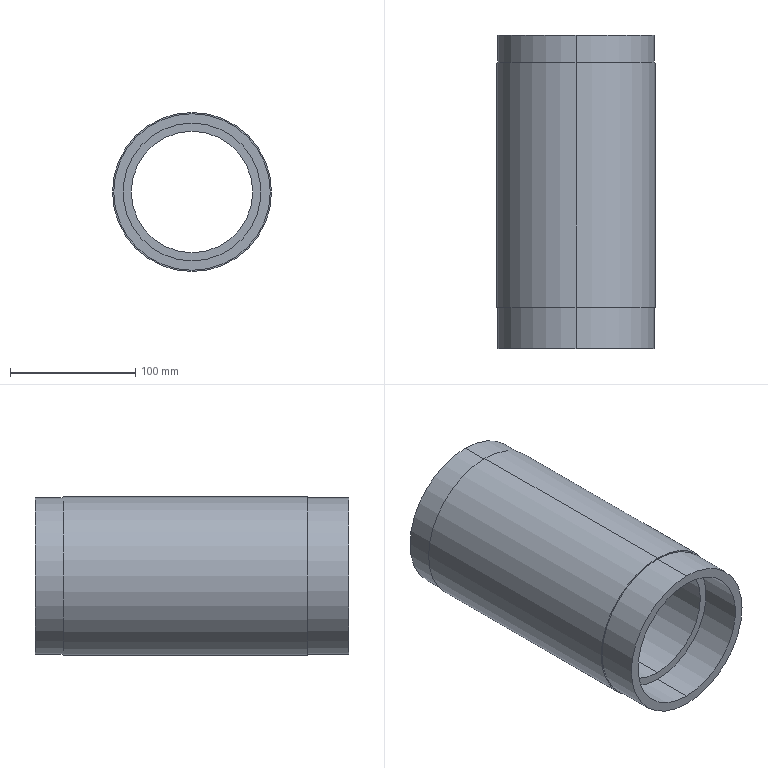Part | SolidWorks | features Revolution 1 | 1 solid | 18 faces | box 127 x 250 x 127 mm | volume 1158206 mm3 | cylinder 12 | plane 6 | commonest cylinder face diameters 110 x4 125 x4 97 x2 127 x2
STEP:
#1=CARTESIAN_POINT('',(0.,33.,-62.5));
#2=VERTEX_POINT('',#1);
#3=CARTESIAN_POINT('',(0.,33.,62.5));
#4=VERTEX_POINT('',#3);
#5=CARTESIAN_POINT('',(0.,33.,0.));
#6=DIRECTION('',(0.,-1.,0.));
#7=DIRECTION('',(0.,0.,-1.));
#8=AXIS2_PLACEMENT_3D('',#5,#6,#7);
#9=CIRCLE('',#8,62.5);
#10=EDGE_CURVE('',#2,#4,#9,.T.);
#11=ORIENTED_EDGE('',*,*,#10,.T.);
#12=CARTESIAN_POINT('',(0.,0.,62.5));
#13=VERTEX_POINT('',#12);
#14=CARTESIAN_POINT('',(0.,0.,62.5));
#15=DIRECTION('',(0.,-1.,0.));
#16=VECTOR('',#15,1000.);
#17=LINE('',#14,#16);
#18=EDGE_CURVE('',#4,#13,#17,.T.);
#19=ORIENTED_EDGE('',*,*,#18,.T.);
#20=CARTESIAN_POINT('',(0.,0.,-62.5));
#21=VERTEX_POINT('',#20);
#22=CARTESIAN_POINT('',(0.,0.,0.));
#23=DIRECTION('',(0.,-1.,0.));
#24=DIRECTION('',(0.,0.,-1.));
#25=AXIS2_PLACEMENT_3D('',#22,#23,#24);
#26=CIRCLE('',#25,62.5);
#27=EDGE_CURVE('',#21,#13,#26,.T.);
#28=ORIENTED_EDGE('',*,*,#27,.F.);
#29=CARTESIAN_POINT('',(0.,0.,-62.5));
#30=DIRECTION('',(0.,-1.,0.));
#31=VECTOR('',#30,1000.);
#32=LINE('',#29,#31);
#33=EDGE_CURVE('',#2,#21,#32,.T.);
#34=ORIENTED_EDGE('',*,*,#33,.F.);
#35=EDGE_LOOP('',(#11,#19,#28,#34));
#36=FACE_OUTER_BOUND('',#35,.T.);
#37=CARTESIAN_POINT('',(0.,0.,0.));
#38=DIRECTION('',(0.,-1.,0.));
#39=DIRECTION('',(0.,0.,-1.));
#40=AXIS2_PLACEMENT_3D('',#37,#38,#39);
#41=CYLINDRICAL_SURFACE('',#40,62.5);
#42=ADVANCED_FACE('',(#36),#41,.T.);
#43=CARTESIAN_POINT('',(0.,228.,-63.5));
#44=VERTEX_POINT('',#43);
#45=CARTESIAN_POINT('',(0.,228.,63.5));
#46=VERTEX_POINT('',#45);
#47=CARTESIAN_POINT('',(0.,228.,0.));
#48=DIRECTION('',(0.,-1.,0.));
#49=DIRECTION('',(0.,0.,-1.));
#50=AXIS2_PLACEMENT_3D('',#47,#48,#49);
#51=CIRCLE('',#50,63.5);
#52=EDGE_CURVE('',#44,#46,#51,.T.);
#53=ORIENTED_EDGE('',*,*,#52,.T.);
#54=CARTESIAN_POINT('',(0.,33.,63.5));
#55=VERTEX_POINT('',#54);
#56=CARTESIAN_POINT('',(0.,0.,63.5));
#57=DIRECTION('',(0.,-1.,0.));
#58=VECTOR('',#57,1000.);
#59=LINE('',#56,#58);
#60=EDGE_CURVE('',#46,#55,#59,.T.);
#61=ORIENTED_EDGE('',*,*,#60,.T.);
#62=CARTESIAN_POINT('',(0.,33.,-63.5));
#63=VERTEX_POINT('',#62);
#64=CARTESIAN_POINT('',(0.,33.,0.));
#65=DIRECTION('',(0.,-1.,0.));
#66=DIRECTION('',(0.,0.,-1.));
#67=AXIS2_PLACEMENT_3D('',#64,#65,#66);
#68=CIRCLE('',#67,63.5);
#69=EDGE_CURVE('',#63,#55,#68,.T.);
#70=ORIENTED_EDGE('',*,*,#69,.F.);
#71=CARTESIAN_POINT('',(0.,0.,-63.5));
#72=DIRECTION('',(0.,-1.,0.));
#73=VECTOR('',#72,1000.);
#74=LINE('',#71,#73);
#75=EDGE_CURVE('',#44,#63,#74,.T.);
#76=ORIENTED_EDGE('',*,*,#75,.F.);
#77=EDGE_LOOP('',(#53,#61,#70,#76));
#78=FACE_OUTER_BOUND('',#77,.T.);
#79=CARTESIAN_POINT('',(0.,0.,0.));
#80=DIRECTION('',(0.,-1.,0.));
#81=DIRECTION('',(0.,0.,-1.));
#82=AXIS2_PLACEMENT_3D('',#79,#80,#81);
#83=CYLINDRICAL_SURFACE('',#82,63.5);
#84=ADVANCED_FACE('',(#78),#83,.T.);
#85=CARTESIAN_POINT('',(0.,250.,-62.5));
#86=VERTEX_POINT('',#85);
#87=CARTESIAN_POINT('',(0.,250.,62.5));
#88=VERTEX_POINT('',#87);
#89=CARTESIAN_POINT('',(0.,250.,0.));
#90=DIRECTION('',(0.,-1.,0.));
#91=DIRECTION('',(0.,0.,-1.));
#92=AXIS2_PLACEMENT_3D('',#89,#90,#91);
#93=CIRCLE('',#92,62.5);
#94=EDGE_CURVE('',#86,#88,#93,.T.);
#95=ORIENTED_EDGE('',*,*,#94,.T.);
#96=CARTESIAN_POINT('',(0.,228.,62.5));
#97=VERTEX_POINT('',#96);
#98=CARTESIAN_POINT('',(0.,0.,62.5));
#99=DIRECTION('',(0.,-1.,0.));
#100=VECTOR('',#99,1000.);
#101=LINE('',#98,#100);
#102=EDGE_CURVE('',#88,#97,#101,.T.);
#103=ORIENTED_EDGE('',*,*,#102,.T.);
#104=CARTESIAN_POINT('',(0.,228.,-62.5));
#105=VERTEX_POINT('',#104);
#106=CARTESIAN_POINT('',(0.,228.,0.));
#107=DIRECTION('',(0.,-1.,0.));
#108=DIRECTION('',(0.,0.,-1.));
#109=AXIS2_PLACEMENT_3D('',#106,#107,#108);
#110=CIRCLE('',#109,62.5);
#111=EDGE_CURVE('',#105,#97,#110,.T.);
#112=ORIENTED_EDGE('',*,*,#111,.F.);
#113=CARTESIAN_POINT('',(0.,0.,-62.5));
#114=DIRECTION('',(0.,-1.,0.));
#115=VECTOR('',#114,1000.);
#116=LINE('',#113,#115);
#117=EDGE_CURVE('',#86,#105,#116,.T.);
#118=ORIENTED_EDGE('',*,*,#117,.F.);
#119=EDGE_LOOP('',(#95,#103,#112,#118));
#120=FACE_OUTER_BOUND('',#119,.T.);
#121=CARTESIAN_POINT('',(0.,0.,0.));
#122=DIRECTION('',(0.,-1.,0.));
#123=DIRECTION('',(0.,0.,-1.));
#124=AXIS2_PLACEMENT_3D('',#121,#122,#123);
#125=CYLINDRICAL_SURFACE('',#124,62.5);
#126=ADVANCED_FACE('',(#120),#125,.T.);
#127=CARTESIAN_POINT('',(0.,250.,55.));
#128=VERTEX_POINT('',#127);
#129=CARTESIAN_POINT('',(0.,250.,-55.));
#130=VERTEX_POINT('',#129);
#131=CARTESIAN_POINT('',(0.,250.,0.));
#132=DIRECTION('',(0.,-1.,0.));
#133=DIRECTION('',(0.,0.,-1.));
#134=AXIS2_PLACEMENT_3D('',#131,#132,#133);
#135=CIRCLE('',#134,55.);
#136=EDGE_CURVE('',#128,#130,#135,.T.);
#137=ORIENTED_EDGE('',*,*,#136,.F.);
#138=CARTESIAN_POINT('',(0.,217.,55.));
#139=VERTEX_POINT('',#138);
#140=CARTESIAN_POINT('',(0.,0.,55.));
#141=DIRECTION('',(0.,-1.,0.));
#142=VECTOR('',#141,1000.);
#143=LINE('',#140,#142);
#144=EDGE_CURVE('',#128,#139,#143,.T.);
#145=ORIENTED_EDGE('',*,*,#144,.T.);
#146=CARTESIAN_POINT('',(0.,217.,-55.));
#147=VERTEX_POINT('',#146);
#148=CARTESIAN_POINT('',(0.,217.,0.));
#149=DIRECTION('',(0.,-1.,0.));
#150=DIRECTION('',(0.,0.,-1.));
#151=AXIS2_PLACEMENT_3D('',#148,#149,#150);
#152=CIRCLE('',#151,55.);
#153=EDGE_CURVE('',#139,#147,#152,.T.);
#154=ORIENTED_EDGE('',*,*,#153,.T.);
#155=CARTESIAN_POINT('',(0.,0.,-55.));
#156=DIRECTION('',(0.,-1.,0.));
#157=VECTOR('',#156,1000.);
#158=LINE('',#155,#157);
#159=EDGE_CURVE('',#130,#147,#158,.T.);
#160=ORIENTED_EDGE('',*,*,#159,.F.);
#161=EDGE_LOOP('',(#137,#145,#154,#160));
#162=FACE_OUTER_BOUND('',#161,.T.);
#163=CARTESIAN_POINT('',(0.,0.,0.));
#164=DIRECTION('',(0.,-1.,0.));
#165=DIRECTION('',(0.,0.,-1.));
#166=AXIS2_PLACEMENT_3D('',#163,#164,#165);
#167=CYLINDRICAL_SURFACE('',#166,55.);
#168=ADVANCED_FACE('',(#162),#167,.F.);
#169=CARTESIAN_POINT('',(0.,217.,48.5));
#170=VERTEX_POINT('',#169);
#171=CARTESIAN_POINT('',(0.,217.,-48.5));
#172=VERTEX_POINT('',#171);
#173=CARTESIAN_POINT('',(0.,217.,0.));
#174=DIRECTION('',(0.,-1.,0.));
#175=DIRECTION('',(0.,0.,-1.));
#176=AXIS2_PLACEMENT_3D('',#173,#174,#175);
#177=CIRCLE('',#176,48.5);
#178=EDGE_CURVE('',#170,#172,#177,.T.);
#179=ORIENTED_EDGE('',*,*,#178,.F.);
#180=CARTESIAN_POINT('',(0.,33.,48.5));
#181=VERTEX_POINT('',#180);
#182=CARTESIAN_POINT('',(0.,0.,48.5));
#183=DIRECTION('',(0.,-1.,0.));
#184=VECTOR('',#183,1000.);
#185=LINE('',#182,#184);
#186=EDGE_CURVE('',#170,#181,#185,.T.);
#187=ORIENTED_EDGE('',*,*,#186,.T.);
#188=CARTESIAN_POINT('',(0.,33.,-48.5));
#189=VERTEX_POINT('',#188);
#190=CARTESIAN_POINT('',(0.,33.,0.));
#191=DIRECTION('',(0.,-1.,0.));
#192=DIRECTION('',(0.,0.,-1.));
#193=AXIS2_PLACEMENT_3D('',#190,#191,#192);
#194=CIRCLE('',#193,48.5);
#195=EDGE_CURVE('',#181,#189,#194,.T.);
#196=ORIENTED_EDGE('',*,*,#195,.T.);
#197=CARTESIAN_POINT('',(0.,0.,-48.5));
#198=DIRECTION('',(0.,-1.,0.));
#199=VECTOR('',#198,1000.);
#200=LINE('',#197,#199);
#201=EDGE_CURVE('',#172,#189,#200,.T.);
#202=ORIENTED_EDGE('',*,*,#201,.F.);
#203=EDGE_LOOP('',(#179,#187,#196,#202));
#204=FACE_OUTER_BOUND('',#203,.T.);
#205=CARTESIAN_POINT('',(0.,0.,0.));
#206=DIRECTION('',(0.,-1.,0.));
#207=DIRECTION('',(0.,0.,-1.));
#208=AXIS2_PLACEMENT_3D('',#205,#206,#207);
#209=CYLINDRICAL_SURFACE('',#208,48.5);
#210=ADVANCED_FACE('',(#204),#209,.F.);
#211=CARTESIAN_POINT('',(0.,33.,55.));
#212=VERTEX_POINT('',#211);
#213=CARTESIAN_POINT('',(0.,33.,-55.));
#214=VERTEX_POINT('',#213);
#215=CARTESIAN_POINT('',(0.,33.,0.));
#216=DIRECTION('',(0.,-1.,0.));
#217=DIRECTION('',(0.,0.,-1.));
#218=AXIS2_PLACEMENT_3D('',#215,#216,#217);
#219=CIRCLE('',#218,55.);
#220=EDGE_CURVE('',#212,#214,#219,.T.);
#221=ORIENTED_EDGE('',*,*,#220,.F.);
#222=CARTESIAN_POINT('',(0.,0.,55.));
#223=VERTEX_POINT('',#222);
#224=CARTESIAN_POINT('',(0.,0.,55.));
#225=DIRECTION('',(0.,-1.,0.));
#226=VECTOR('',#225,1000.);
#227=LINE('',#224,#226);
#228=EDGE_CURVE('',#212,#223,#227,.T.);
#229=ORIENTED_EDGE('',*,*,#228,.T.);
#230=CARTESIAN_POINT('',(0.,0.,-55.));
#231=VERTEX_POINT('',#230);
#232=CARTESIAN_POINT('',(0.,0.,0.));
#233=DIRECTION('',(0.,-1.,0.));
#234=DIRECTION('',(0.,0.,-1.));
#235=AXIS2_PLACEMENT_3D('',#232,#233,#234);
#236=CIRCLE('',#235,55.);
#237=EDGE_CURVE('',#223,#231,#236,.T.);
#238=ORIENTED_EDGE('',*,*,#237,.T.);
#239=CARTESIAN_POINT('',(0.,0.,-55.));
#240=DIRECTION('',(0.,-1.,0.));
#241=VECTOR('',#240,1000.);
#242=LINE('',#239,#241);
#243=EDGE_CURVE('',#214,#231,#242,.T.);
#244=ORIENTED_EDGE('',*,*,#243,.F.);
#245=EDGE_LOOP('',(#221,#229,#238,#244));
#246=FACE_OUTER_BOUND('',#245,.T.);
#247=CARTESIAN_POINT('',(0.,0.,0.));
#248=DIRECTION('',(0.,-1.,0.));
#249=DIRECTION('',(0.,0.,-1.));
#250=AXIS2_PLACEMENT_3D('',#247,#248,#249);
#251=CYLINDRICAL_SURFACE('',#250,55.);
#252=ADVANCED_FACE('',(#246),#251,.F.);
#253=ORIENTED_EDGE('',*,*,#27,.T.);
#254=CARTESIAN_POINT('',(0.,0.,0.));
#255=DIRECTION('',(0.,-1.,0.));
#256=DIRECTION('',(0.,0.,-1.));
#257=AXIS2_PLACEMENT_3D('',#254,#255,#256);
#258=CIRCLE('',#257,62.5);
#259=EDGE_CURVE('',#13,#21,#258,.T.);
#260=ORIENTED_EDGE('',*,*,#259,.T.);
#261=EDGE_LOOP('',(#253,#260));
#262=FACE_OUTER_BOUND('',#261,.T.);
#263=CARTESIAN_POINT('',(0.,0.,0.));
#264=DIRECTION('',(0.,-1.,0.));
#265=DIRECTION('',(0.,0.,-1.));
#266=AXIS2_PLACEMENT_3D('',#263,#264,#265);
#267=CIRCLE('',#266,55.);
#268=EDGE_CURVE('',#231,#223,#267,.T.);
#269=ORIENTED_EDGE('',*,*,#268,.F.);
#270=ORIENTED_EDGE('',*,*,#237,.F.);
#271=EDGE_LOOP('',(#269,#270));
#272=FACE_BOUND('',#271,.T.);
#273=CARTESIAN_POINT('',(62.5,0.,0.));
#274=DIRECTION('',(0.,-1.,0.));
#275=DIRECTION('',(0.,0.,-1.));
#276=AXIS2_PLACEMENT_3D('',#273,#274,#275);
#277=PLANE('',#276);
#278=ADVANCED_FACE('',(#262,#272),#277,.T.);
#279=ORIENTED_EDGE('',*,*,#228,.F.);
#280=CARTESIAN_POINT('',(0.,33.,0.));
#281=DIRECTION('',(0.,-1.,0.));
#282=DIRECTION('',(0.,0.,-1.));
#283=AXIS2_PLACEMENT_3D('',#280,#281,#282);
#284=CIRCLE('',#283,55.);
#285=EDGE_CURVE('',#214,#212,#284,.T.);
#286=ORIENTED_EDGE('',*,*,#285,.F.);
#287=ORIENTED_EDGE('',*,*,#243,.T.);
#288=ORIENTED_EDGE('',*,*,#268,.T.);
#289=EDGE_LOOP('',(#279,#286,#287,#288));
#290=FACE_OUTER_BOUND('',#289,.T.);
#291=CARTESIAN_POINT('',(0.,0.,0.));
#292=DIRECTION('',(0.,-1.,0.));
#293=DIRECTION('',(0.,0.,-1.));
#294=AXIS2_PLACEMENT_3D('',#291,#292,#293);
#295=CYLINDRICAL_SURFACE('',#294,55.);
#296=ADVANCED_FACE('',(#290),#295,.F.);
#297=ORIENTED_EDGE('',*,*,#285,.T.);
#298=ORIENTED_EDGE('',*,*,#220,.T.);
#299=EDGE_LOOP('',(#297,#298));
#300=FACE_OUTER_BOUND('',#299,.T.);
#301=CARTESIAN_POINT('',(0.,33.,0.));
#302=DIRECTION('',(0.,-1.,0.));
#303=DIRECTION('',(0.,0.,-1.));
#304=AXIS2_PLACEMENT_3D('',#301,#302,#303);
#305=CIRCLE('',#304,48.5);
#306=EDGE_CURVE('',#189,#181,#305,.T.);
#307=ORIENTED_EDGE('',*,*,#306,.F.);
#308=ORIENTED_EDGE('',*,*,#195,.F.);
#309=EDGE_LOOP('',(#307,#308));
#310=FACE_BOUND('',#309,.T.);
#311=CARTESIAN_POINT('',(55.,33.,0.));
#312=DIRECTION('',(0.,-1.,0.));
#313=DIRECTION('',(0.,0.,-1.));
#314=AXIS2_PLACEMENT_3D('',#311,#312,#313);
#315=PLANE('',#314);
#316=ADVANCED_FACE('',(#300,#310),#315,.T.);
#317=ORIENTED_EDGE('',*,*,#186,.F.);
#318=CARTESIAN_POINT('',(0.,217.,0.));
#319=DIRECTION('',(0.,-1.,0.));
#320=DIRECTION('',(0.,0.,-1.));
#321=AXIS2_PLACEMENT_3D('',#318,#319,#320);
#322=CIRCLE('',#321,48.5);
#323=EDGE_CURVE('',#172,#170,#322,.T.);
#324=ORIENTED_EDGE('',*,*,#323,.F.);
#325=ORIENTED_EDGE('',*,*,#201,.T.);
#326=ORIENTED_EDGE('',*,*,#306,.T.);
#327=EDGE_LOOP('',(#317,#324,#325,#326));
#328=FACE_OUTER_BOUND('',#327,.T.);
#329=CARTESIAN_POINT('',(0.,0.,0.));
#330=DIRECTION('',(0.,-1.,0.));
#331=DIRECTION('',(0.,0.,-1.));
#332=AXIS2_PLACEMENT_3D('',#329,#330,#331);
#333=CYLINDRICAL_SURFACE('',#332,48.5);
#334=ADVANCED_FACE('',(#328),#333,.F.);
#335=ORIENTED_EDGE('',*,*,#323,.T.);
#336=ORIENTED_EDGE('',*,*,#178,.T.);
#337=EDGE_LOOP('',(#335,#336));
#338=FACE_BOUND('',#337,.T.);
#339=CARTESIAN_POINT('',(0.,217.,0.));
#340=DIRECTION('',(0.,-1.,0.));
#341=DIRECTION('',(0.,0.,-1.));
#342=AXIS2_PLACEMENT_3D('',#339,#340,#341);
#343=CIRCLE('',#342,55.);
#344=EDGE_CURVE('',#147,#139,#343,.T.);
#345=ORIENTED_EDGE('',*,*,#344,.F.);
#346=ORIENTED_EDGE('',*,*,#153,.F.);
#347=EDGE_LOOP('',(#345,#346));
#348=FACE_OUTER_BOUND('',#347,.T.);
#349=CARTESIAN_POINT('',(48.5,217.,0.));
#350=DIRECTION('',(0.,1.,0.));
#351=DIRECTION('',(0.,0.,1.));
#352=AXIS2_PLACEMENT_3D('',#349,#350,#351);
#353=PLANE('',#352);
#354=ADVANCED_FACE('',(#338,#348),#353,.T.);
#355=ORIENTED_EDGE('',*,*,#144,.F.);
#356=CARTESIAN_POINT('',(0.,250.,0.));
#357=DIRECTION('',(0.,-1.,0.));
#358=DIRECTION('',(0.,0.,-1.));
#359=AXIS2_PLACEMENT_3D('',#356,#357,#358);
#360=CIRCLE('',#359,55.);
#361=EDGE_CURVE('',#130,#128,#360,.T.);
#362=ORIENTED_EDGE('',*,*,#361,.F.);
#363=ORIENTED_EDGE('',*,*,#159,.T.);
#364=ORIENTED_EDGE('',*,*,#344,.T.);
#365=EDGE_LOOP('',(#355,#362,#363,#364));
#366=FACE_OUTER_BOUND('',#365,.T.);
#367=CARTESIAN_POINT('',(0.,0.,0.));
#368=DIRECTION('',(0.,-1.,0.));
#369=DIRECTION('',(0.,0.,-1.));
#370=AXIS2_PLACEMENT_3D('',#367,#368,#369);
#371=CYLINDRICAL_SURFACE('',#370,55.);
#372=ADVANCED_FACE('',(#366),#371,.F.);
#373=ORIENTED_EDGE('',*,*,#361,.T.);
#374=ORIENTED_EDGE('',*,*,#136,.T.);
#375=EDGE_LOOP('',(#373,#374));
#376=FACE_BOUND('',#375,.T.);
#377=ORIENTED_EDGE('',*,*,#94,.F.);
#378=CARTESIAN_POINT('',(0.,250.,0.));
#379=DIRECTION('',(0.,-1.,0.));
#380=DIRECTION('',(0.,0.,-1.));
#381=AXIS2_PLACEMENT_3D('',#378,#379,#380);
#382=CIRCLE('',#381,62.5);
#383=EDGE_CURVE('',#88,#86,#382,.T.);
#384=ORIENTED_EDGE('',*,*,#383,.F.);
#385=EDGE_LOOP('',(#377,#384));
#386=FACE_OUTER_BOUND('',#385,.T.);
#387=CARTESIAN_POINT('',(55.,250.,0.));
#388=DIRECTION('',(0.,1.,0.));
#389=DIRECTION('',(0.,0.,1.));
#390=AXIS2_PLACEMENT_3D('',#387,#388,#389);
#391=PLANE('',#390);
#392=ADVANCED_FACE('',(#376,#386),#391,.T.);
#393=ORIENTED_EDGE('',*,*,#102,.F.);
#394=ORIENTED_EDGE('',*,*,#383,.T.);
#395=ORIENTED_EDGE('',*,*,#117,.T.);
#396=CARTESIAN_POINT('',(0.,228.,0.));
#397=DIRECTION('',(0.,-1.,0.));
#398=DIRECTION('',(0.,0.,-1.));
#399=AXIS2_PLACEMENT_3D('',#396,#397,#398);
#400=CIRCLE('',#399,62.5);
#401=EDGE_CURVE('',#97,#105,#400,.T.);
#402=ORIENTED_EDGE('',*,*,#401,.F.);
#403=EDGE_LOOP('',(#393,#394,#395,#402));
#404=FACE_OUTER_BOUND('',#403,.T.);
#405=CARTESIAN_POINT('',(0.,0.,0.));
#406=DIRECTION('',(0.,-1.,0.));
#407=DIRECTION('',(0.,0.,-1.));
#408=AXIS2_PLACEMENT_3D('',#405,#406,#407);
#409=CYLINDRICAL_SURFACE('',#408,62.5);
#410=ADVANCED_FACE('',(#404),#409,.T.);
#411=ORIENTED_EDGE('',*,*,#111,.T.);
#412=ORIENTED_EDGE('',*,*,#401,.T.);
#413=EDGE_LOOP('',(#411,#412));
#414=FACE_BOUND('',#413,.T.);
#415=ORIENTED_EDGE('',*,*,#52,.F.);
#416=CARTESIAN_POINT('',(0.,228.,0.));
#417=DIRECTION('',(0.,-1.,0.));
#418=DIRECTION('',(0.,0.,-1.));
#419=AXIS2_PLACEMENT_3D('',#416,#417,#418);
#420=CIRCLE('',#419,63.5);
#421=EDGE_CURVE('',#46,#44,#420,.T.);
#422=ORIENTED_EDGE('',*,*,#421,.F.);
#423=EDGE_LOOP('',(#415,#422));
#424=FACE_OUTER_BOUND('',#423,.T.);
#425=CARTESIAN_POINT('',(62.5,228.,0.));
#426=DIRECTION('',(0.,1.,0.));
#427=DIRECTION('',(0.,0.,1.));
#428=AXIS2_PLACEMENT_3D('',#425,#426,#427);
#429=PLANE('',#428);
#430=ADVANCED_FACE('',(#414,#424),#429,.T.);
#431=ORIENTED_EDGE('',*,*,#60,.F.);
#432=ORIENTED_EDGE('',*,*,#421,.T.);
#433=ORIENTED_EDGE('',*,*,#75,.T.);
#434=CARTESIAN_POINT('',(0.,33.,0.));
#435=DIRECTION('',(0.,-1.,0.));
#436=DIRECTION('',(0.,0.,-1.));
#437=AXIS2_PLACEMENT_3D('',#434,#435,#436);
#438=CIRCLE('',#437,63.5);
#439=EDGE_CURVE('',#55,#63,#438,.T.);
#440=ORIENTED_EDGE('',*,*,#439,.F.);
#441=EDGE_LOOP('',(#431,#432,#433,#440));
#442=FACE_OUTER_BOUND('',#441,.T.);
#443=CARTESIAN_POINT('',(0.,0.,0.));
#444=DIRECTION('',(0.,-1.,0.));
#445=DIRECTION('',(0.,0.,-1.));
#446=AXIS2_PLACEMENT_3D('',#443,#444,#445);
#447=CYLINDRICAL_SURFACE('',#446,63.5);
#448=ADVANCED_FACE('',(#442),#447,.T.);
#449=ORIENTED_EDGE('',*,*,#69,.T.);
#450=ORIENTED_EDGE('',*,*,#439,.T.);
#451=EDGE_LOOP('',(#449,#450));
#452=FACE_OUTER_BOUND('',#451,.T.);
#453=ORIENTED_EDGE('',*,*,#10,.F.);
#454=CARTESIAN_POINT('',(0.,33.,0.));
#455=DIRECTION('',(0.,-1.,0.));
#456=DIRECTION('',(0.,0.,-1.));
#457=AXIS2_PLACEMENT_3D('',#454,#455,#456);
#458=CIRCLE('',#457,62.5);
#459=EDGE_CURVE('',#4,#2,#458,.T.);
#460=ORIENTED_EDGE('',*,*,#459,.F.);
#461=EDGE_LOOP('',(#453,#460));
#462=FACE_BOUND('',#461,.T.);
#463=CARTESIAN_POINT('',(63.5,33.,0.));
#464=DIRECTION('',(0.,-1.,0.));
#465=DIRECTION('',(0.,0.,-1.));
#466=AXIS2_PLACEMENT_3D('',#463,#464,#465);
#467=PLANE('',#466);
#468=ADVANCED_FACE('',(#452,#462),#467,.T.);
#469=ORIENTED_EDGE('',*,*,#18,.F.);
#470=ORIENTED_EDGE('',*,*,#459,.T.);
#471=ORIENTED_EDGE('',*,*,#33,.T.);
#472=ORIENTED_EDGE('',*,*,#259,.F.);
#473=EDGE_LOOP('',(#469,#470,#471,#472));
#474=FACE_OUTER_BOUND('',#473,.T.);
#475=CARTESIAN_POINT('',(0.,0.,0.));
#476=DIRECTION('',(0.,-1.,0.));
#477=DIRECTION('',(0.,0.,-1.));
#478=AXIS2_PLACEMENT_3D('',#475,#476,#477);
#479=CYLINDRICAL_SURFACE('',#478,62.5);
#480=ADVANCED_FACE('',(#474),#479,.T.);
#481=CLOSED_SHELL('',(#42,#84,#126,#168,#210,#252,#278,#296,#316,#334,#354,#372,#392,#410,#430,#448,#468,#480));
#482=MANIFOLD_SOLID_BREP('',#481);
#483=CARTESIAN_POINT('',(0.,0.,0.));
#484=DIRECTION('',(0.,0.,1.));
#485=DIRECTION('',(1.,0.,0.));
#486=AXIS2_PLACEMENT_3D('',#483,#484,#485);
#487=(LENGTH_UNIT()NAMED_UNIT(*)SI_UNIT(.MILLI.,.METRE.));
#488=UNCERTAINTY_MEASURE_WITH_UNIT(LENGTH_MEASURE(0.00001),#487,'','');
#489=(NAMED_UNIT(*)PLANE_ANGLE_UNIT()SI_UNIT($,.RADIAN.));
#490=(NAMED_UNIT(*)SI_UNIT($,.STERADIAN.)SOLID_ANGLE_UNIT());
#491=(GEOMETRIC_REPRESENTATION_CONTEXT(3)GLOBAL_UNCERTAINTY_ASSIGNED_CONTEXT((#488))GLOBAL_UNIT_ASSIGNED_CONTEXT((#487,#489,#490))REPRESENTATION_CONTEXT('',''));
#492=ADVANCED_BREP_SHAPE_REPRESENTATION('',(#482,#486),#491);